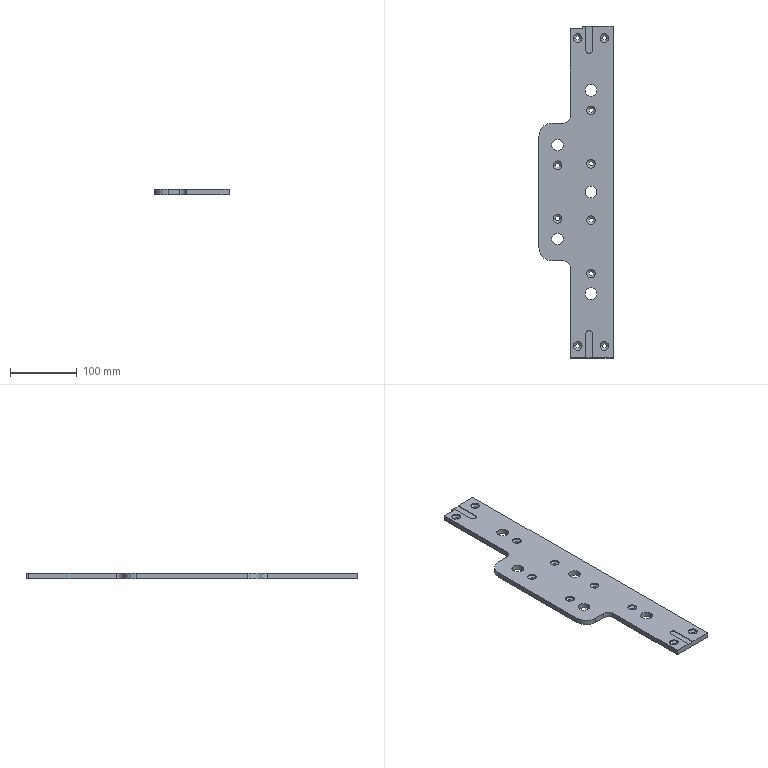Part | Creo | 1 solid | 94 faces | box 111 x 496 x 8 mm | volume 313901 mm3 | cylinder 56 | cone 20 | plane 18 | commonest cylinder face diameters 6.6 x20 13 x20 17.4 x10 10 x2 20 x2 40 x2